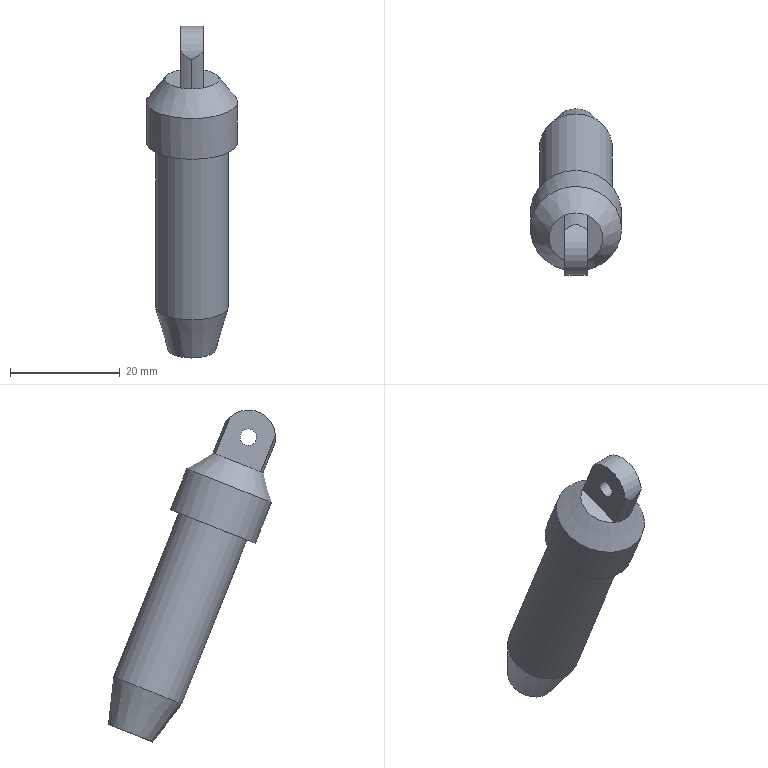Part | STEP file | Cut-Extrude2 | 1 solid | 19 faces | box 16.64 x 30.437 x 60.503 mm | volume 5800 mm3 | cylinder 9 | plane 8 | cone 2 | commonest cylinder face diameters 9.8 x3 3 x2 9.4 x1 9.919 x1 13.32 x1 16.64 x1